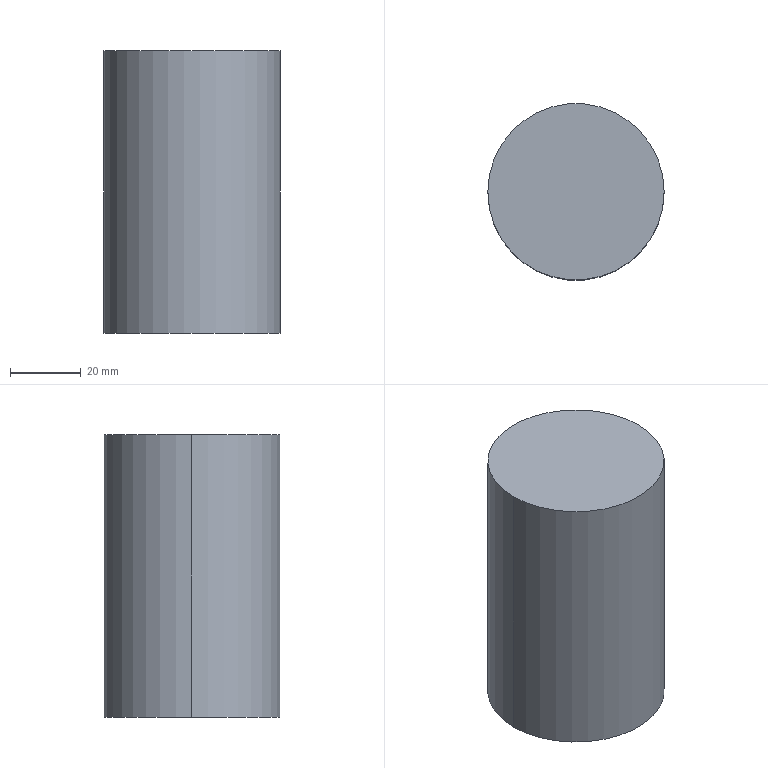Part | SolidWorks | features Extrusion 1 | 1 solid | 4 faces | box 50 x 50 x 80 mm | volume 157080 mm3 | cylinder 2 | plane 2 | commonest cylinder face diameters 50 x2
STEP:
#1=CARTESIAN_POINT('',(25.,0.,-80.));
#2=VERTEX_POINT('',#1);
#3=CARTESIAN_POINT('',(-25.,0.,-80.));
#4=VERTEX_POINT('',#3);
#5=CARTESIAN_POINT('',(0.,0.,-80.));
#6=DIRECTION('',(0.,0.,1.));
#7=DIRECTION('',(1.,0.,0.));
#8=AXIS2_PLACEMENT_3D('',#5,#6,#7);
#9=CIRCLE('',#8,25.);
#10=EDGE_CURVE('',#2,#4,#9,.T.);
#11=ORIENTED_EDGE('',*,*,#10,.T.);
#12=CARTESIAN_POINT('',(-25.,0.,0.));
#13=VERTEX_POINT('',#12);
#14=CARTESIAN_POINT('',(-25.,0.,-80.));
#15=DIRECTION('',(0.,0.,1.));
#16=VECTOR('',#15,1000.);
#17=LINE('',#14,#16);
#18=EDGE_CURVE('',#4,#13,#17,.T.);
#19=ORIENTED_EDGE('',*,*,#18,.T.);
#20=CARTESIAN_POINT('',(25.,0.,0.));
#21=VERTEX_POINT('',#20);
#22=CARTESIAN_POINT('',(0.,0.,0.));
#23=DIRECTION('',(0.,0.,1.));
#24=DIRECTION('',(1.,0.,0.));
#25=AXIS2_PLACEMENT_3D('',#22,#23,#24);
#26=CIRCLE('',#25,25.);
#27=EDGE_CURVE('',#21,#13,#26,.T.);
#28=ORIENTED_EDGE('',*,*,#27,.F.);
#29=CARTESIAN_POINT('',(25.,0.,-80.));
#30=DIRECTION('',(0.,0.,1.));
#31=VECTOR('',#30,1000.);
#32=LINE('',#29,#31);
#33=EDGE_CURVE('',#2,#21,#32,.T.);
#34=ORIENTED_EDGE('',*,*,#33,.F.);
#35=EDGE_LOOP('',(#11,#19,#28,#34));
#36=FACE_OUTER_BOUND('',#35,.T.);
#37=CARTESIAN_POINT('',(0.,0.,-80.));
#38=DIRECTION('',(0.,0.,1.));
#39=DIRECTION('',(1.,0.,0.));
#40=AXIS2_PLACEMENT_3D('',#37,#38,#39);
#41=CYLINDRICAL_SURFACE('',#40,25.);
#42=ADVANCED_FACE('',(#36),#41,.T.);
#43=ORIENTED_EDGE('',*,*,#18,.F.);
#44=CARTESIAN_POINT('',(0.,0.,-80.));
#45=DIRECTION('',(0.,0.,1.));
#46=DIRECTION('',(1.,0.,0.));
#47=AXIS2_PLACEMENT_3D('',#44,#45,#46);
#48=CIRCLE('',#47,25.);
#49=EDGE_CURVE('',#4,#2,#48,.T.);
#50=ORIENTED_EDGE('',*,*,#49,.T.);
#51=ORIENTED_EDGE('',*,*,#33,.T.);
#52=CARTESIAN_POINT('',(0.,0.,0.));
#53=DIRECTION('',(0.,0.,1.));
#54=DIRECTION('',(1.,0.,0.));
#55=AXIS2_PLACEMENT_3D('',#52,#53,#54);
#56=CIRCLE('',#55,25.);
#57=EDGE_CURVE('',#13,#21,#56,.T.);
#58=ORIENTED_EDGE('',*,*,#57,.F.);
#59=EDGE_LOOP('',(#43,#50,#51,#58));
#60=FACE_OUTER_BOUND('',#59,.T.);
#61=CARTESIAN_POINT('',(0.,0.,-80.));
#62=DIRECTION('',(0.,0.,1.));
#63=DIRECTION('',(1.,0.,0.));
#64=AXIS2_PLACEMENT_3D('',#61,#62,#63);
#65=CYLINDRICAL_SURFACE('',#64,25.);
#66=ADVANCED_FACE('',(#60),#65,.T.);
#67=ORIENTED_EDGE('',*,*,#10,.F.);
#68=ORIENTED_EDGE('',*,*,#49,.F.);
#69=EDGE_LOOP('',(#67,#68));
#70=FACE_OUTER_BOUND('',#69,.T.);
#71=CARTESIAN_POINT('',(0.,0.,-80.));
#72=DIRECTION('',(0.,0.,1.));
#73=DIRECTION('',(1.,0.,0.));
#74=AXIS2_PLACEMENT_3D('',#71,#72,#73);
#75=PLANE('',#74);
#76=ADVANCED_FACE('',(#70),#75,.F.);
#77=ORIENTED_EDGE('',*,*,#27,.T.);
#78=ORIENTED_EDGE('',*,*,#57,.T.);
#79=EDGE_LOOP('',(#77,#78));
#80=FACE_OUTER_BOUND('',#79,.T.);
#81=CARTESIAN_POINT('',(0.,0.,0.));
#82=DIRECTION('',(0.,0.,1.));
#83=DIRECTION('',(1.,0.,0.));
#84=AXIS2_PLACEMENT_3D('',#81,#82,#83);
#85=PLANE('',#84);
#86=ADVANCED_FACE('',(#80),#85,.T.);
#87=CLOSED_SHELL('',(#42,#66,#76,#86));
#88=MANIFOLD_SOLID_BREP('',#87);
#89=CARTESIAN_POINT('',(0.,0.,0.));
#90=DIRECTION('',(0.,0.,1.));
#91=DIRECTION('',(1.,0.,0.));
#92=AXIS2_PLACEMENT_3D('',#89,#90,#91);
#93=(LENGTH_UNIT()NAMED_UNIT(*)SI_UNIT(.MILLI.,.METRE.));
#94=UNCERTAINTY_MEASURE_WITH_UNIT(LENGTH_MEASURE(0.00001),#93,'','');
#95=(NAMED_UNIT(*)PLANE_ANGLE_UNIT()SI_UNIT($,.RADIAN.));
#96=(NAMED_UNIT(*)SI_UNIT($,.STERADIAN.)SOLID_ANGLE_UNIT());
#97=(GEOMETRIC_REPRESENTATION_CONTEXT(3)GLOBAL_UNCERTAINTY_ASSIGNED_CONTEXT((#94))GLOBAL_UNIT_ASSIGNED_CONTEXT((#93,#95,#96))REPRESENTATION_CONTEXT('',''));
#98=ADVANCED_BREP_SHAPE_REPRESENTATION('',(#88,#92),#97);